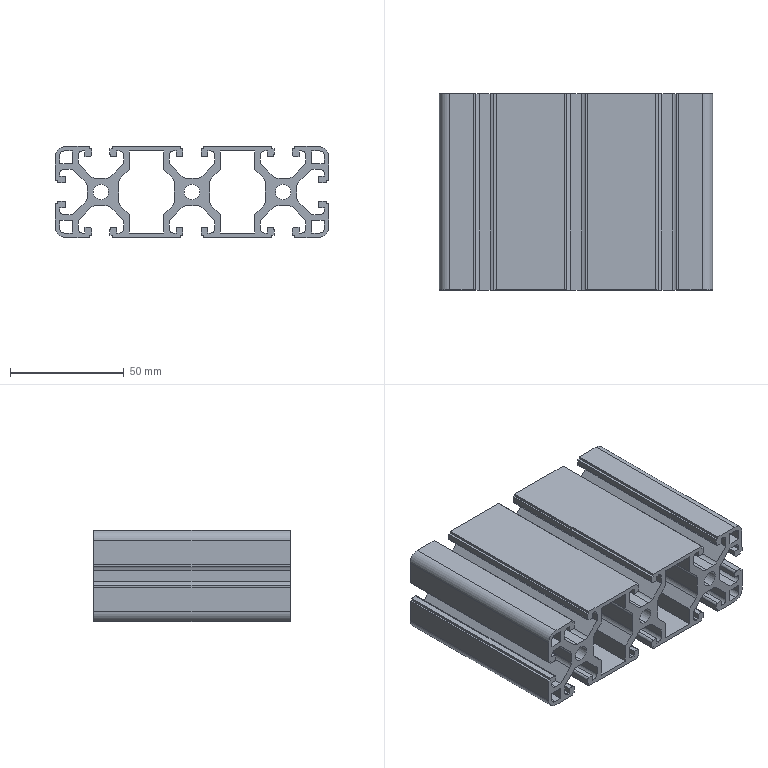Part | STEP file | Vibratory feeder support_Default<machined> | 1 solid | 260 faces | box 120 x 86.083 x 40 mm | volume 137280 mm3 | plane 190 | cylinder 70 | commonest cylinder face diameters 6 x24 4 x20 2 x16 6.8 x6 9 x4